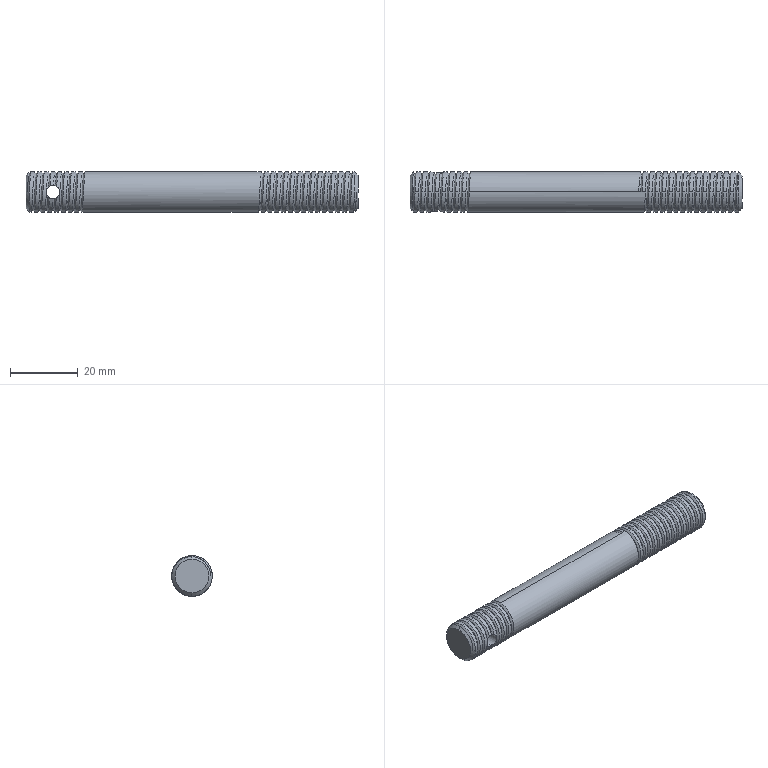Part | SolidWorks | features Helix 2, SweepCut 2, Chamfer 1, ICE 1, Revolution 1 | 1 solid | 72 faces | box 98 x 12 x 12 mm | volume 10688 mm3 | cylinder 52 | spline 14 | plane 4 | cone 2 | commonest cylinder face diameters 12 x50 4 x2